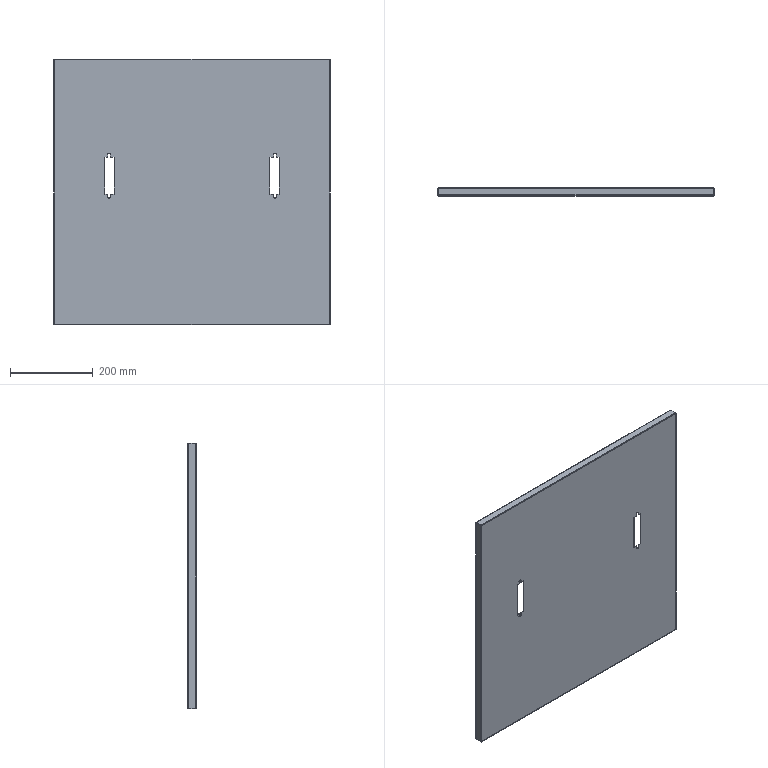Part | STEP file | JBJ-P-1011-05b | 1 solid | 106 faces | box 668 x 20 x 643 mm | volume 606779 mm3 | plane 58 | cylinder 32 | spline 16 | commonest cylinder face diameters 4 x12 2 x8 4.4 x8 7 x4